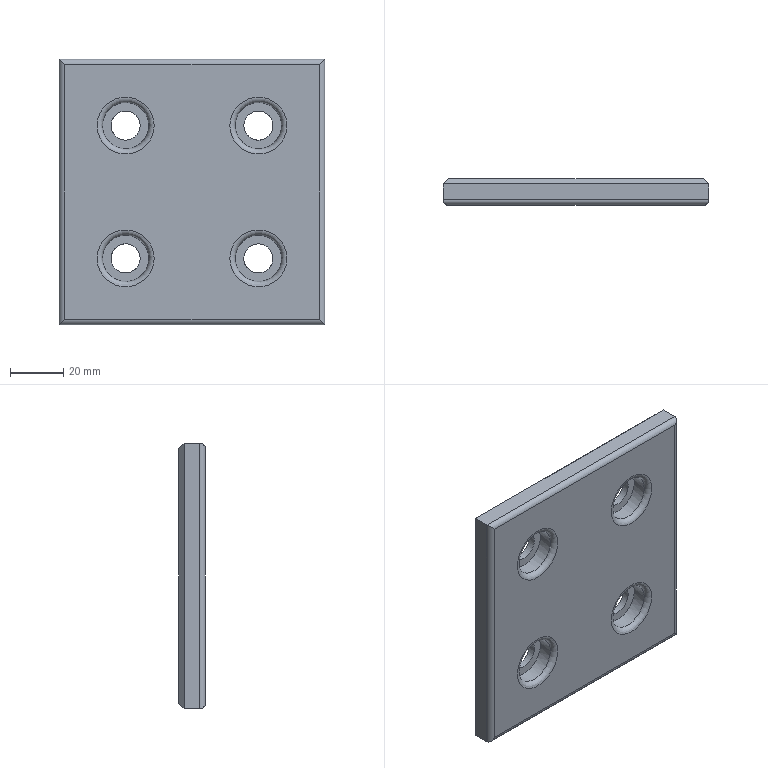Part | NX | features MAIN_BODY 2 | 1 solid | 30 faces | box 100 x 10 x 100 mm | volume 90622 mm3 | plane 14 | cylinder 12 | torus 4 | commonest cylinder face diameters 4 x4 11 x4 17.5 x4
STEP:
#1=CARTESIAN_POINT('',(-666.,240.,-150.5));
#2=VERTEX_POINT('',#1);
#3=CARTESIAN_POINT('',(-570.,240.,-150.5));
#4=VERTEX_POINT('',#3);
#5=CARTESIAN_POINT('',(-568.,240.,-150.5));
#6=DIRECTION('',(-1.,0.,0.));
#7=VECTOR('',#6,1000.);
#8=LINE('',#5,#7);
#9=EDGE_CURVE('',#2,#4,#8,.F.);
#10=ORIENTED_EDGE('',*,*,#9,.T.);
#11=CARTESIAN_POINT('',(-570.,240.,-54.5));
#12=VERTEX_POINT('',#11);
#13=CARTESIAN_POINT('',(-570.,240.,-152.5));
#14=DIRECTION('',(0.,0.,-1.));
#15=VECTOR('',#14,1000.);
#16=LINE('',#13,#15);
#17=EDGE_CURVE('',#4,#12,#16,.F.);
#18=ORIENTED_EDGE('',*,*,#17,.T.);
#19=CARTESIAN_POINT('',(-666.,240.,-54.5));
#20=VERTEX_POINT('',#19);
#21=CARTESIAN_POINT('',(-568.,240.,-54.5));
#22=DIRECTION('',(1.,0.,0.));
#23=VECTOR('',#22,1000.);
#24=LINE('',#21,#23);
#25=EDGE_CURVE('',#12,#20,#24,.F.);
#26=ORIENTED_EDGE('',*,*,#25,.T.);
#27=CARTESIAN_POINT('',(-666.,240.,-152.5));
#28=DIRECTION('',(0.,0.,1.));
#29=VECTOR('',#28,1000.);
#30=LINE('',#27,#29);
#31=EDGE_CURVE('',#20,#2,#30,.F.);
#32=ORIENTED_EDGE('',*,*,#31,.T.);
#33=EDGE_LOOP('',(#10,#18,#26,#32));
#34=FACE_BOUND('',#33,.T.);
#35=CARTESIAN_POINT('',(-582.25,240.,-127.5));
#36=VERTEX_POINT('',#35);
#37=CARTESIAN_POINT('',(-593.,240.,-127.5));
#38=DIRECTION('',(0.,-1.,0.));
#39=DIRECTION('',(1.,0.,0.));
#40=AXIS2_PLACEMENT_3D('',#37,#38,#39);
#41=CIRCLE('',#40,10.75);
#42=EDGE_CURVE('',#36,#36,#41,.F.);
#43=ORIENTED_EDGE('',*,*,#42,.T.);
#44=EDGE_LOOP('',(#43));
#45=FACE_BOUND('',#44,.T.);
#46=CARTESIAN_POINT('',(-582.25,240.,-77.5));
#47=VERTEX_POINT('',#46);
#48=CARTESIAN_POINT('',(-593.,240.,-77.5));
#49=DIRECTION('',(0.,-1.,0.));
#50=DIRECTION('',(1.,0.,0.));
#51=AXIS2_PLACEMENT_3D('',#48,#49,#50);
#52=CIRCLE('',#51,10.75);
#53=EDGE_CURVE('',#47,#47,#52,.F.);
#54=ORIENTED_EDGE('',*,*,#53,.T.);
#55=EDGE_LOOP('',(#54));
#56=FACE_BOUND('',#55,.T.);
#57=CARTESIAN_POINT('',(-632.25,240.,-77.5));
#58=VERTEX_POINT('',#57);
#59=CARTESIAN_POINT('',(-643.,240.,-77.5));
#60=DIRECTION('',(0.,-1.,0.));
#61=DIRECTION('',(1.,0.,0.));
#62=AXIS2_PLACEMENT_3D('',#59,#60,#61);
#63=CIRCLE('',#62,10.75);
#64=EDGE_CURVE('',#58,#58,#63,.F.);
#65=ORIENTED_EDGE('',*,*,#64,.T.);
#66=EDGE_LOOP('',(#65));
#67=FACE_BOUND('',#66,.T.);
#68=CARTESIAN_POINT('',(-632.25,240.,-127.5));
#69=VERTEX_POINT('',#68);
#70=CARTESIAN_POINT('',(-643.,240.,-127.5));
#71=DIRECTION('',(0.,-1.,0.));
#72=DIRECTION('',(1.,0.,0.));
#73=AXIS2_PLACEMENT_3D('',#70,#71,#72);
#74=CIRCLE('',#73,10.75);
#75=EDGE_CURVE('',#69,#69,#74,.F.);
#76=ORIENTED_EDGE('',*,*,#75,.T.);
#77=EDGE_LOOP('',(#76));
#78=FACE_BOUND('',#77,.T.);
#79=CARTESIAN_POINT('',(-568.,240.,-152.5));
#80=DIRECTION('',(0.,-1.,0.));
#81=DIRECTION('',(1.,0.,0.));
#82=AXIS2_PLACEMENT_3D('',#79,#80,#81);
#83=PLANE('',#82);
#84=ADVANCED_FACE('',(#34,#45,#56,#67,#78),#83,.T.);
#85=CARTESIAN_POINT('',(-643.,250.,-83.));
#86=VERTEX_POINT('',#85);
#87=CARTESIAN_POINT('',(-643.,250.,-77.5));
#88=DIRECTION('',(0.,-1.,0.));
#89=DIRECTION('',(0.,0.,-1.));
#90=AXIS2_PLACEMENT_3D('',#87,#88,#89);
#91=CIRCLE('',#90,5.5);
#92=EDGE_CURVE('',#86,#86,#91,.T.);
#93=ORIENTED_EDGE('',*,*,#92,.F.);
#94=EDGE_LOOP('',(#93));
#95=FACE_BOUND('',#94,.T.);
#96=CARTESIAN_POINT('',(-637.5,247.3,-77.5));
#97=VERTEX_POINT('',#96);
#98=CARTESIAN_POINT('',(-643.,247.3,-77.5));
#99=DIRECTION('',(0.,-1.,0.));
#100=DIRECTION('',(1.,0.,0.));
#101=AXIS2_PLACEMENT_3D('',#98,#99,#100);
#102=CIRCLE('',#101,5.5);
#103=EDGE_CURVE('',#97,#97,#102,.T.);
#104=ORIENTED_EDGE('',*,*,#103,.T.);
#105=EDGE_LOOP('',(#104));
#106=FACE_BOUND('',#105,.T.);
#107=CARTESIAN_POINT('',(-643.,230.,-77.5));
#108=DIRECTION('',(0.,1.,0.));
#109=DIRECTION('',(-1.,0.,0.));
#110=AXIS2_PLACEMENT_3D('',#107,#108,#109);
#111=CYLINDRICAL_SURFACE('',#110,5.5);
#112=ADVANCED_FACE('',(#95,#106),#111,.F.);
#113=CARTESIAN_POINT('',(-593.,250.,-122.));
#114=VERTEX_POINT('',#113);
#115=CARTESIAN_POINT('',(-593.,250.,-127.5));
#116=DIRECTION('',(0.,-1.,0.));
#117=DIRECTION('',(0.,0.,1.));
#118=AXIS2_PLACEMENT_3D('',#115,#116,#117);
#119=CIRCLE('',#118,5.5);
#120=EDGE_CURVE('',#114,#114,#119,.T.);
#121=ORIENTED_EDGE('',*,*,#120,.F.);
#122=EDGE_LOOP('',(#121));
#123=FACE_BOUND('',#122,.T.);
#124=CARTESIAN_POINT('',(-587.5,247.3,-127.5));
#125=VERTEX_POINT('',#124);
#126=CARTESIAN_POINT('',(-593.,247.3,-127.5));
#127=DIRECTION('',(0.,-1.,0.));
#128=DIRECTION('',(1.,0.,0.));
#129=AXIS2_PLACEMENT_3D('',#126,#127,#128);
#130=CIRCLE('',#129,5.5);
#131=EDGE_CURVE('',#125,#125,#130,.T.);
#132=ORIENTED_EDGE('',*,*,#131,.T.);
#133=EDGE_LOOP('',(#132));
#134=FACE_BOUND('',#133,.T.);
#135=CARTESIAN_POINT('',(-593.,230.,-127.5));
#136=DIRECTION('',(0.,1.,0.));
#137=DIRECTION('',(-1.,0.,0.));
#138=AXIS2_PLACEMENT_3D('',#135,#136,#137);
#139=CYLINDRICAL_SURFACE('',#138,5.5);
#140=ADVANCED_FACE('',(#123,#134),#139,.F.);
#141=CARTESIAN_POINT('',(-666.,250.,-54.5));
#142=VERTEX_POINT('',#141);
#143=CARTESIAN_POINT('',(-570.,250.,-54.5));
#144=VERTEX_POINT('',#143);
#145=CARTESIAN_POINT('',(-568.,250.,-54.5));
#146=DIRECTION('',(1.,0.,0.));
#147=VECTOR('',#146,1000.);
#148=LINE('',#145,#147);
#149=EDGE_CURVE('',#142,#144,#148,.T.);
#150=ORIENTED_EDGE('',*,*,#149,.T.);
#151=CARTESIAN_POINT('',(-570.,250.,-150.5));
#152=VERTEX_POINT('',#151);
#153=CARTESIAN_POINT('',(-570.,250.,-152.5));
#154=DIRECTION('',(0.,0.,-1.));
#155=VECTOR('',#154,1000.);
#156=LINE('',#153,#155);
#157=EDGE_CURVE('',#144,#152,#156,.T.);
#158=ORIENTED_EDGE('',*,*,#157,.T.);
#159=CARTESIAN_POINT('',(-666.,250.,-150.5));
#160=VERTEX_POINT('',#159);
#161=CARTESIAN_POINT('',(-668.,250.,-150.5));
#162=DIRECTION('',(-1.,0.,0.));
#163=VECTOR('',#162,1000.);
#164=LINE('',#161,#163);
#165=EDGE_CURVE('',#152,#160,#164,.T.);
#166=ORIENTED_EDGE('',*,*,#165,.T.);
#167=CARTESIAN_POINT('',(-666.,250.,-52.5));
#168=DIRECTION('',(0.,0.,1.));
#169=VECTOR('',#168,1000.);
#170=LINE('',#167,#169);
#171=EDGE_CURVE('',#160,#142,#170,.T.);
#172=ORIENTED_EDGE('',*,*,#171,.T.);
#173=EDGE_LOOP('',(#150,#158,#166,#172));
#174=FACE_BOUND('',#173,.T.);
#175=CARTESIAN_POINT('',(-643.,250.,-122.));
#176=VERTEX_POINT('',#175);
#177=CARTESIAN_POINT('',(-643.,250.,-127.5));
#178=DIRECTION('',(0.,1.,0.));
#179=DIRECTION('',(0.,0.,1.));
#180=AXIS2_PLACEMENT_3D('',#177,#178,#179);
#181=CIRCLE('',#180,5.5);
#182=EDGE_CURVE('',#176,#176,#181,.T.);
#183=ORIENTED_EDGE('',*,*,#182,.F.);
#184=EDGE_LOOP('',(#183));
#185=FACE_BOUND('',#184,.T.);
#186=ORIENTED_EDGE('',*,*,#92,.T.);
#187=EDGE_LOOP('',(#186));
#188=FACE_BOUND('',#187,.T.);
#189=CARTESIAN_POINT('',(-593.,250.,-83.));
#190=VERTEX_POINT('',#189);
#191=CARTESIAN_POINT('',(-593.,250.,-77.5));
#192=DIRECTION('',(0.,1.,0.));
#193=DIRECTION('',(0.,0.,-1.));
#194=AXIS2_PLACEMENT_3D('',#191,#192,#193);
#195=CIRCLE('',#194,5.5);
#196=EDGE_CURVE('',#190,#190,#195,.T.);
#197=ORIENTED_EDGE('',*,*,#196,.F.);
#198=EDGE_LOOP('',(#197));
#199=FACE_BOUND('',#198,.T.);
#200=ORIENTED_EDGE('',*,*,#120,.T.);
#201=EDGE_LOOP('',(#200));
#202=FACE_BOUND('',#201,.T.);
#203=CARTESIAN_POINT('',(-568.,250.,-152.5));
#204=DIRECTION('',(0.,-1.,0.));
#205=DIRECTION('',(1.,0.,0.));
#206=AXIS2_PLACEMENT_3D('',#203,#204,#205);
#207=PLANE('',#206);
#208=ADVANCED_FACE('',(#174,#185,#188,#199,#202),#207,.F.);
#209=CARTESIAN_POINT('',(-668.,242.,-152.5));
#210=VERTEX_POINT('',#209);
#211=CARTESIAN_POINT('',(-668.,248.,-152.5));
#212=VERTEX_POINT('',#211);
#213=CARTESIAN_POINT('',(-668.,240.,-152.5));
#214=DIRECTION('',(0.,1.,0.));
#215=VECTOR('',#214,1000.);
#216=LINE('',#213,#215);
#217=EDGE_CURVE('',#210,#212,#216,.T.);
#218=ORIENTED_EDGE('',*,*,#217,.T.);
#219=CARTESIAN_POINT('',(-568.,248.,-152.5));
#220=VERTEX_POINT('',#219);
#221=CARTESIAN_POINT('',(-568.,248.,-152.5));
#222=DIRECTION('',(1.,0.,0.));
#223=VECTOR('',#222,1000.);
#224=LINE('',#221,#223);
#225=EDGE_CURVE('',#212,#220,#224,.T.);
#226=ORIENTED_EDGE('',*,*,#225,.T.);
#227=CARTESIAN_POINT('',(-568.,242.,-152.5));
#228=VERTEX_POINT('',#227);
#229=CARTESIAN_POINT('',(-568.,240.,-152.5));
#230=DIRECTION('',(0.,1.,0.));
#231=VECTOR('',#230,1000.);
#232=LINE('',#229,#231);
#233=EDGE_CURVE('',#228,#220,#232,.T.);
#234=ORIENTED_EDGE('',*,*,#233,.F.);
#235=CARTESIAN_POINT('',(-568.,242.,-152.5));
#236=DIRECTION('',(-1.,0.,0.));
#237=VECTOR('',#236,1000.);
#238=LINE('',#235,#237);
#239=EDGE_CURVE('',#228,#210,#238,.T.);
#240=ORIENTED_EDGE('',*,*,#239,.T.);
#241=EDGE_LOOP('',(#218,#226,#234,#240));
#242=FACE_BOUND('',#241,.T.);
#243=CARTESIAN_POINT('',(-568.,240.,-152.5));
#244=DIRECTION('',(0.,0.,-1.));
#245=DIRECTION('',(1.,0.,0.));
#246=AXIS2_PLACEMENT_3D('',#243,#244,#245);
#247=PLANE('',#246);
#248=ADVANCED_FACE('',(#242),#247,.T.);
#249=CARTESIAN_POINT('',(-668.,242.,-52.5));
#250=VERTEX_POINT('',#249);
#251=CARTESIAN_POINT('',(-668.,248.,-52.5));
#252=VERTEX_POINT('',#251);
#253=CARTESIAN_POINT('',(-668.,240.,-52.5));
#254=DIRECTION('',(0.,1.,0.));
#255=VECTOR('',#254,1000.);
#256=LINE('',#253,#255);
#257=EDGE_CURVE('',#250,#252,#256,.T.);
#258=ORIENTED_EDGE('',*,*,#257,.T.);
#259=CARTESIAN_POINT('',(-668.,248.,-152.5));
#260=DIRECTION('',(0.,0.,-1.));
#261=VECTOR('',#260,1000.);
#262=LINE('',#259,#261);
#263=EDGE_CURVE('',#252,#212,#262,.T.);
#264=ORIENTED_EDGE('',*,*,#263,.T.);
#265=ORIENTED_EDGE('',*,*,#217,.F.);
#266=CARTESIAN_POINT('',(-668.,242.,-152.5));
#267=DIRECTION('',(0.,0.,1.));
#268=VECTOR('',#267,1000.);
#269=LINE('',#266,#268);
#270=EDGE_CURVE('',#210,#250,#269,.T.);
#271=ORIENTED_EDGE('',*,*,#270,.T.);
#272=EDGE_LOOP('',(#258,#264,#265,#271));
#273=FACE_BOUND('',#272,.T.);
#274=CARTESIAN_POINT('',(-668.,240.,-152.5));
#275=DIRECTION('',(-1.,0.,0.));
#276=DIRECTION('',(0.,0.,-1.));
#277=AXIS2_PLACEMENT_3D('',#274,#275,#276);
#278=PLANE('',#277);
#279=ADVANCED_FACE('',(#273),#278,.T.);
#280=CARTESIAN_POINT('',(-568.,242.,-52.5));
#281=VERTEX_POINT('',#280);
#282=CARTESIAN_POINT('',(-568.,248.,-52.5));
#283=VERTEX_POINT('',#282);
#284=CARTESIAN_POINT('',(-568.,240.,-52.5));
#285=DIRECTION('',(0.,1.,0.));
#286=VECTOR('',#285,1000.);
#287=LINE('',#284,#286);
#288=EDGE_CURVE('',#281,#283,#287,.T.);
#289=ORIENTED_EDGE('',*,*,#288,.T.);
#290=CARTESIAN_POINT('',(-668.,248.,-52.5));
#291=DIRECTION('',(-1.,0.,0.));
#292=VECTOR('',#291,1000.);
#293=LINE('',#290,#292);
#294=EDGE_CURVE('',#283,#252,#293,.T.);
#295=ORIENTED_EDGE('',*,*,#294,.T.);
#296=ORIENTED_EDGE('',*,*,#257,.F.);
#297=CARTESIAN_POINT('',(-668.,242.,-52.5));
#298=DIRECTION('',(1.,0.,0.));
#299=VECTOR('',#298,1000.);
#300=LINE('',#297,#299);
#301=EDGE_CURVE('',#250,#281,#300,.T.);
#302=ORIENTED_EDGE('',*,*,#301,.T.);
#303=EDGE_LOOP('',(#289,#295,#296,#302));
#304=FACE_BOUND('',#303,.T.);
#305=CARTESIAN_POINT('',(-668.,240.,-52.5));
#306=DIRECTION('',(0.,0.,1.));
#307=DIRECTION('',(-1.,0.,0.));
#308=AXIS2_PLACEMENT_3D('',#305,#306,#307);
#309=PLANE('',#308);
#310=ADVANCED_FACE('',(#304),#309,.T.);
#311=ORIENTED_EDGE('',*,*,#233,.T.);
#312=CARTESIAN_POINT('',(-568.,248.,-52.5));
#313=DIRECTION('',(0.,0.,1.));
#314=VECTOR('',#313,1000.);
#315=LINE('',#312,#314);
#316=EDGE_CURVE('',#220,#283,#315,.T.);
#317=ORIENTED_EDGE('',*,*,#316,.T.);
#318=ORIENTED_EDGE('',*,*,#288,.F.);
#319=CARTESIAN_POINT('',(-568.,242.,-52.5));
#320=DIRECTION('',(0.,0.,-1.));
#321=VECTOR('',#320,1000.);
#322=LINE('',#319,#321);
#323=EDGE_CURVE('',#281,#228,#322,.T.);
#324=ORIENTED_EDGE('',*,*,#323,.T.);
#325=EDGE_LOOP('',(#311,#317,#318,#324));
#326=FACE_BOUND('',#325,.T.);
#327=CARTESIAN_POINT('',(-568.,240.,-52.5));
#328=DIRECTION('',(1.,0.,0.));
#329=DIRECTION('',(0.,0.,1.));
#330=AXIS2_PLACEMENT_3D('',#327,#328,#329);
#331=PLANE('',#330);
#332=ADVANCED_FACE('',(#326),#331,.T.);
#333=CARTESIAN_POINT('',(-598.5,247.3,-77.5));
#334=VERTEX_POINT('',#333);
#335=CARTESIAN_POINT('',(-593.,247.3,-77.5));
#336=DIRECTION('',(0.,1.,0.));
#337=DIRECTION('',(-1.,0.,0.));
#338=AXIS2_PLACEMENT_3D('',#335,#336,#337);
#339=CIRCLE('',#338,5.5);
#340=EDGE_CURVE('',#334,#334,#339,.F.);
#341=ORIENTED_EDGE('',*,*,#340,.T.);
#342=EDGE_LOOP('',(#341));
#343=FACE_BOUND('',#342,.T.);
#344=ORIENTED_EDGE('',*,*,#196,.T.);
#345=EDGE_LOOP('',(#344));
#346=FACE_BOUND('',#345,.T.);
#347=CARTESIAN_POINT('',(-593.,230.,-77.5));
#348=DIRECTION('',(0.,1.,0.));
#349=DIRECTION('',(-1.,0.,0.));
#350=AXIS2_PLACEMENT_3D('',#347,#348,#349);
#351=CYLINDRICAL_SURFACE('',#350,5.5);
#352=ADVANCED_FACE('',(#343,#346),#351,.F.);
#353=CARTESIAN_POINT('',(-648.5,247.3,-127.5));
#354=VERTEX_POINT('',#353);
#355=CARTESIAN_POINT('',(-643.,247.3,-127.5));
#356=DIRECTION('',(0.,1.,0.));
#357=DIRECTION('',(-1.,0.,0.));
#358=AXIS2_PLACEMENT_3D('',#355,#356,#357);
#359=CIRCLE('',#358,5.5);
#360=EDGE_CURVE('',#354,#354,#359,.F.);
#361=ORIENTED_EDGE('',*,*,#360,.T.);
#362=EDGE_LOOP('',(#361));
#363=FACE_BOUND('',#362,.T.);
#364=ORIENTED_EDGE('',*,*,#182,.T.);
#365=EDGE_LOOP('',(#364));
#366=FACE_BOUND('',#365,.T.);
#367=CARTESIAN_POINT('',(-643.,230.,-127.5));
#368=DIRECTION('',(0.,1.,0.));
#369=DIRECTION('',(-1.,0.,0.));
#370=AXIS2_PLACEMENT_3D('',#367,#368,#369);
#371=CYLINDRICAL_SURFACE('',#370,5.5);
#372=ADVANCED_FACE('',(#363,#366),#371,.F.);
#373=CARTESIAN_POINT('',(-584.25,242.,-127.5));
#374=VERTEX_POINT('',#373);
#375=CARTESIAN_POINT('',(-593.,242.,-127.5));
#376=DIRECTION('',(0.,-1.,0.));
#377=DIRECTION('',(1.,0.,0.));
#378=AXIS2_PLACEMENT_3D('',#375,#376,#377);
#379=CIRCLE('',#378,8.75);
#380=EDGE_CURVE('',#374,#374,#379,.T.);
#381=ORIENTED_EDGE('',*,*,#380,.T.);
#382=EDGE_LOOP('',(#381));
#383=FACE_BOUND('',#382,.T.);
#384=CARTESIAN_POINT('',(-593.,247.3,-118.75));
#385=VERTEX_POINT('',#384);
#386=CARTESIAN_POINT('',(-593.,247.3,-127.5));
#387=DIRECTION('',(0.,-1.,0.));
#388=DIRECTION('',(0.,0.,1.));
#389=AXIS2_PLACEMENT_3D('',#386,#387,#388);
#390=CIRCLE('',#389,8.75);
#391=EDGE_CURVE('',#385,#385,#390,.T.);
#392=ORIENTED_EDGE('',*,*,#391,.F.);
#393=EDGE_LOOP('',(#392));
#394=FACE_BOUND('',#393,.T.);
#395=CARTESIAN_POINT('',(-593.,220.,-127.5));
#396=DIRECTION('',(0.,1.,0.));
#397=DIRECTION('',(-1.,0.,0.));
#398=AXIS2_PLACEMENT_3D('',#395,#396,#397);
#399=CYLINDRICAL_SURFACE('',#398,8.75);
#400=ADVANCED_FACE('',(#383,#394),#399,.F.);
#401=ORIENTED_EDGE('',*,*,#131,.F.);
#402=EDGE_LOOP('',(#401));
#403=FACE_BOUND('',#402,.T.);
#404=ORIENTED_EDGE('',*,*,#391,.T.);
#405=EDGE_LOOP('',(#404));
#406=FACE_BOUND('',#405,.T.);
#407=CARTESIAN_POINT('',(-593.,247.3,-127.5));
#408=DIRECTION('',(0.,-1.,0.));
#409=DIRECTION('',(1.,0.,0.));
#410=AXIS2_PLACEMENT_3D('',#407,#408,#409);
#411=PLANE('',#410);
#412=ADVANCED_FACE('',(#403,#406),#411,.T.);
#413=CARTESIAN_POINT('',(-643.,247.3,-118.75));
#414=VERTEX_POINT('',#413);
#415=CARTESIAN_POINT('',(-643.,247.3,-127.5));
#416=DIRECTION('',(0.,1.,0.));
#417=DIRECTION('',(0.,0.,1.));
#418=AXIS2_PLACEMENT_3D('',#415,#416,#417);
#419=CIRCLE('',#418,8.75);
#420=EDGE_CURVE('',#414,#414,#419,.T.);
#421=ORIENTED_EDGE('',*,*,#420,.F.);
#422=EDGE_LOOP('',(#421));
#423=FACE_BOUND('',#422,.T.);
#424=ORIENTED_EDGE('',*,*,#360,.F.);
#425=EDGE_LOOP('',(#424));
#426=FACE_BOUND('',#425,.T.);
#427=CARTESIAN_POINT('',(-643.,247.3,-127.5));
#428=DIRECTION('',(0.,1.,0.));
#429=DIRECTION('',(-1.,0.,0.));
#430=AXIS2_PLACEMENT_3D('',#427,#428,#429);
#431=PLANE('',#430);
#432=ADVANCED_FACE('',(#423,#426),#431,.F.);
#433=CARTESIAN_POINT('',(-634.25,242.,-127.5));
#434=VERTEX_POINT('',#433);
#435=CARTESIAN_POINT('',(-643.,242.,-127.5));
#436=DIRECTION('',(0.,-1.,0.));
#437=DIRECTION('',(1.,0.,0.));
#438=AXIS2_PLACEMENT_3D('',#435,#436,#437);
#439=CIRCLE('',#438,8.75);
#440=EDGE_CURVE('',#434,#434,#439,.T.);
#441=ORIENTED_EDGE('',*,*,#440,.T.);
#442=EDGE_LOOP('',(#441));
#443=FACE_BOUND('',#442,.T.);
#444=ORIENTED_EDGE('',*,*,#420,.T.);
#445=EDGE_LOOP('',(#444));
#446=FACE_BOUND('',#445,.T.);
#447=CARTESIAN_POINT('',(-643.,220.,-127.5));
#448=DIRECTION('',(0.,1.,0.));
#449=DIRECTION('',(-1.,0.,0.));
#450=AXIS2_PLACEMENT_3D('',#447,#448,#449);
#451=CYLINDRICAL_SURFACE('',#450,8.75);
#452=ADVANCED_FACE('',(#443,#446),#451,.F.);
#453=CARTESIAN_POINT('',(-593.,247.3,-86.25));
#454=VERTEX_POINT('',#453);
#455=CARTESIAN_POINT('',(-593.,247.3,-77.5));
#456=DIRECTION('',(0.,1.,0.));
#457=DIRECTION('',(0.,0.,-1.));
#458=AXIS2_PLACEMENT_3D('',#455,#456,#457);
#459=CIRCLE('',#458,8.75);
#460=EDGE_CURVE('',#454,#454,#459,.T.);
#461=ORIENTED_EDGE('',*,*,#460,.F.);
#462=EDGE_LOOP('',(#461));
#463=FACE_BOUND('',#462,.T.);
#464=ORIENTED_EDGE('',*,*,#340,.F.);
#465=EDGE_LOOP('',(#464));
#466=FACE_BOUND('',#465,.T.);
#467=CARTESIAN_POINT('',(-593.,247.3,-77.5));
#468=DIRECTION('',(0.,1.,0.));
#469=DIRECTION('',(-1.,0.,0.));
#470=AXIS2_PLACEMENT_3D('',#467,#468,#469);
#471=PLANE('',#470);
#472=ADVANCED_FACE('',(#463,#466),#471,.F.);
#473=CARTESIAN_POINT('',(-584.25,242.,-77.5));
#474=VERTEX_POINT('',#473);
#475=CARTESIAN_POINT('',(-593.,242.,-77.5));
#476=DIRECTION('',(0.,-1.,0.));
#477=DIRECTION('',(1.,0.,0.));
#478=AXIS2_PLACEMENT_3D('',#475,#476,#477);
#479=CIRCLE('',#478,8.75);
#480=EDGE_CURVE('',#474,#474,#479,.T.);
#481=ORIENTED_EDGE('',*,*,#480,.T.);
#482=EDGE_LOOP('',(#481));
#483=FACE_BOUND('',#482,.T.);
#484=ORIENTED_EDGE('',*,*,#460,.T.);
#485=EDGE_LOOP('',(#484));
#486=FACE_BOUND('',#485,.T.);
#487=CARTESIAN_POINT('',(-593.,220.,-77.5));
#488=DIRECTION('',(0.,1.,0.));
#489=DIRECTION('',(-1.,0.,0.));
#490=AXIS2_PLACEMENT_3D('',#487,#488,#489);
#491=CYLINDRICAL_SURFACE('',#490,8.75);
#492=ADVANCED_FACE('',(#483,#486),#491,.F.);
#493=CARTESIAN_POINT('',(-634.25,242.,-77.5));
#494=VERTEX_POINT('',#493);
#495=CARTESIAN_POINT('',(-643.,242.,-77.5));
#496=DIRECTION('',(0.,-1.,0.));
#497=DIRECTION('',(1.,0.,0.));
#498=AXIS2_PLACEMENT_3D('',#495,#496,#497);
#499=CIRCLE('',#498,8.75);
#500=EDGE_CURVE('',#494,#494,#499,.T.);
#501=ORIENTED_EDGE('',*,*,#500,.T.);
#502=EDGE_LOOP('',(#501));
#503=FACE_BOUND('',#502,.T.);
#504=CARTESIAN_POINT('',(-643.,247.3,-86.25));
#505=VERTEX_POINT('',#504);
#506=CARTESIAN_POINT('',(-643.,247.3,-77.5));
#507=DIRECTION('',(0.,-1.,0.));
#508=DIRECTION('',(0.,0.,-1.));
#509=AXIS2_PLACEMENT_3D('',#506,#507,#508);
#510=CIRCLE('',#509,8.75);
#511=EDGE_CURVE('',#505,#505,#510,.T.);
#512=ORIENTED_EDGE('',*,*,#511,.F.);
#513=EDGE_LOOP('',(#512));
#514=FACE_BOUND('',#513,.T.);
#515=CARTESIAN_POINT('',(-643.,220.,-77.5));
#516=DIRECTION('',(0.,1.,0.));
#517=DIRECTION('',(-1.,0.,0.));
#518=AXIS2_PLACEMENT_3D('',#515,#516,#517);
#519=CYLINDRICAL_SURFACE('',#518,8.75);
#520=ADVANCED_FACE('',(#503,#514),#519,.F.);
#521=ORIENTED_EDGE('',*,*,#103,.F.);
#522=EDGE_LOOP('',(#521));
#523=FACE_BOUND('',#522,.T.);
#524=ORIENTED_EDGE('',*,*,#511,.T.);
#525=EDGE_LOOP('',(#524));
#526=FACE_BOUND('',#525,.T.);
#527=CARTESIAN_POINT('',(-643.,247.3,-77.5));
#528=DIRECTION('',(0.,-1.,0.));
#529=DIRECTION('',(1.,0.,0.));
#530=AXIS2_PLACEMENT_3D('',#527,#528,#529);
#531=PLANE('',#530);
#532=ADVANCED_FACE('',(#523,#526),#531,.T.);
#533=CARTESIAN_POINT('',(-666.,242.,-150.5));
#534=DIRECTION('',(-0.7071,0.,0.7071));
#535=DIRECTION('',(0.7071,0.,0.7071));
#536=AXIS2_PLACEMENT_3D('',#533,#534,#535);
#537=ELLIPSE('',#536,2.828,2.);
#538=EDGE_CURVE('',#2,#210,#537,.F.);
#539=ORIENTED_EDGE('',*,*,#538,.F.);
#540=ORIENTED_EDGE('',*,*,#31,.F.);
#541=CARTESIAN_POINT('',(-666.,242.,-54.5));
#542=DIRECTION('',(0.7071,0.,0.7071));
#543=DIRECTION('',(-0.7071,0.,0.7071));
#544=AXIS2_PLACEMENT_3D('',#541,#542,#543);
#545=ELLIPSE('',#544,2.828,2.);
#546=EDGE_CURVE('',#250,#20,#545,.T.);
#547=ORIENTED_EDGE('',*,*,#546,.F.);
#548=ORIENTED_EDGE('',*,*,#270,.F.);
#549=EDGE_LOOP('',(#539,#540,#547,#548));
#550=FACE_BOUND('',#549,.T.);
#551=CARTESIAN_POINT('',(-666.,242.,-152.5));
#552=DIRECTION('',(0.,0.,1.));
#553=DIRECTION('',(-1.,0.,0.));
#554=AXIS2_PLACEMENT_3D('',#551,#552,#553);
#555=CYLINDRICAL_SURFACE('',#554,2.);
#556=ADVANCED_FACE('',(#550),#555,.T.);
#557=ORIENTED_EDGE('',*,*,#546,.T.);
#558=ORIENTED_EDGE('',*,*,#25,.F.);
#559=CARTESIAN_POINT('',(-570.,242.,-54.5));
#560=DIRECTION('',(0.7071,0.,-0.7071));
#561=DIRECTION('',(0.7071,0.,0.7071));
#562=AXIS2_PLACEMENT_3D('',#559,#560,#561);
#563=ELLIPSE('',#562,2.828,2.);
#564=EDGE_CURVE('',#281,#12,#563,.T.);
#565=ORIENTED_EDGE('',*,*,#564,.F.);
#566=ORIENTED_EDGE('',*,*,#301,.F.);
#567=EDGE_LOOP('',(#557,#558,#565,#566));
#568=FACE_BOUND('',#567,.T.);
#569=CARTESIAN_POINT('',(-668.,242.,-54.5));
#570=DIRECTION('',(1.,0.,0.));
#571=DIRECTION('',(0.,0.,1.));
#572=AXIS2_PLACEMENT_3D('',#569,#570,#571);
#573=CYLINDRICAL_SURFACE('',#572,2.);
#574=ADVANCED_FACE('',(#568),#573,.T.);
#575=ORIENTED_EDGE('',*,*,#538,.T.);
#576=ORIENTED_EDGE('',*,*,#239,.F.);
#577=CARTESIAN_POINT('',(-570.,242.,-150.5));
#578=DIRECTION('',(-0.7071,0.,-0.7071));
#579=DIRECTION('',(-0.7071,0.,0.7071));
#580=AXIS2_PLACEMENT_3D('',#577,#578,#579);
#581=ELLIPSE('',#580,2.828,2.);
#582=EDGE_CURVE('',#4,#228,#581,.F.);
#583=ORIENTED_EDGE('',*,*,#582,.F.);
#584=ORIENTED_EDGE('',*,*,#9,.F.);
#585=EDGE_LOOP('',(#575,#576,#583,#584));
#586=FACE_BOUND('',#585,.T.);
#587=CARTESIAN_POINT('',(-568.,242.,-150.5));
#588=DIRECTION('',(-1.,0.,0.));
#589=DIRECTION('',(0.,0.,-1.));
#590=AXIS2_PLACEMENT_3D('',#587,#588,#589);
#591=CYLINDRICAL_SURFACE('',#590,2.);
#592=ADVANCED_FACE('',(#586),#591,.T.);
#593=ORIENTED_EDGE('',*,*,#564,.T.);
#594=ORIENTED_EDGE('',*,*,#17,.F.);
#595=ORIENTED_EDGE('',*,*,#582,.T.);
#596=ORIENTED_EDGE('',*,*,#323,.F.);
#597=EDGE_LOOP('',(#593,#594,#595,#596));
#598=FACE_BOUND('',#597,.T.);
#599=CARTESIAN_POINT('',(-570.,242.,-52.5));
#600=DIRECTION('',(0.,0.,-1.));
#601=DIRECTION('',(1.,0.,0.));
#602=AXIS2_PLACEMENT_3D('',#599,#600,#601);
#603=CYLINDRICAL_SURFACE('',#602,2.);
#604=ADVANCED_FACE('',(#598),#603,.T.);
#605=ORIENTED_EDGE('',*,*,#380,.F.);
#606=EDGE_LOOP('',(#605));
#607=FACE_BOUND('',#606,.T.);
#608=ORIENTED_EDGE('',*,*,#42,.F.);
#609=EDGE_LOOP('',(#608));
#610=FACE_BOUND('',#609,.T.);
#611=CARTESIAN_POINT('',(-593.,242.,-127.5));
#612=DIRECTION('',(0.,-1.,0.));
#613=DIRECTION('',(1.,0.,0.));
#614=AXIS2_PLACEMENT_3D('',#611,#612,#613);
#615=TOROIDAL_SURFACE('',#614,10.75,2.);
#616=ADVANCED_FACE('',(#607,#610),#615,.T.);
#617=ORIENTED_EDGE('',*,*,#53,.F.);
#618=EDGE_LOOP('',(#617));
#619=FACE_BOUND('',#618,.T.);
#620=ORIENTED_EDGE('',*,*,#480,.F.);
#621=EDGE_LOOP('',(#620));
#622=FACE_BOUND('',#621,.T.);
#623=CARTESIAN_POINT('',(-593.,242.,-77.5));
#624=DIRECTION('',(0.,-1.,0.));
#625=DIRECTION('',(1.,0.,0.));
#626=AXIS2_PLACEMENT_3D('',#623,#624,#625);
#627=TOROIDAL_SURFACE('',#626,10.75,2.);
#628=ADVANCED_FACE('',(#619,#622),#627,.T.);
#629=ORIENTED_EDGE('',*,*,#500,.F.);
#630=EDGE_LOOP('',(#629));
#631=FACE_BOUND('',#630,.T.);
#632=ORIENTED_EDGE('',*,*,#64,.F.);
#633=EDGE_LOOP('',(#632));
#634=FACE_BOUND('',#633,.T.);
#635=CARTESIAN_POINT('',(-643.,242.,-77.5));
#636=DIRECTION('',(0.,-1.,0.));
#637=DIRECTION('',(1.,0.,0.));
#638=AXIS2_PLACEMENT_3D('',#635,#636,#637);
#639=TOROIDAL_SURFACE('',#638,10.75,2.);
#640=ADVANCED_FACE('',(#631,#634),#639,.T.);
#641=ORIENTED_EDGE('',*,*,#75,.F.);
#642=EDGE_LOOP('',(#641));
#643=FACE_BOUND('',#642,.T.);
#644=ORIENTED_EDGE('',*,*,#440,.F.);
#645=EDGE_LOOP('',(#644));
#646=FACE_BOUND('',#645,.T.);
#647=CARTESIAN_POINT('',(-643.,242.,-127.5));
#648=DIRECTION('',(0.,-1.,0.));
#649=DIRECTION('',(1.,0.,0.));
#650=AXIS2_PLACEMENT_3D('',#647,#648,#649);
#651=TOROIDAL_SURFACE('',#650,10.75,2.);
#652=ADVANCED_FACE('',(#643,#646),#651,.T.);
#653=CARTESIAN_POINT('',(-666.667,249.333,-151.167));
#654=DIRECTION('',(-0.5774,-0.5774,-0.5774));
#655=VECTOR('',#654,1000.);
#656=LINE('',#653,#655);
#657=EDGE_CURVE('',#212,#160,#656,.F.);
#658=ORIENTED_EDGE('',*,*,#657,.F.);
#659=ORIENTED_EDGE('',*,*,#263,.F.);
#660=CARTESIAN_POINT('',(-633.333,282.667,-87.167));
#661=DIRECTION('',(-0.5774,-0.5774,0.5774));
#662=VECTOR('',#661,1000.);
#663=LINE('',#660,#662);
#664=EDGE_CURVE('',#142,#252,#663,.T.);
#665=ORIENTED_EDGE('',*,*,#664,.F.);
#666=ORIENTED_EDGE('',*,*,#171,.F.);
#667=EDGE_LOOP('',(#658,#659,#665,#666));
#668=FACE_BOUND('',#667,.T.);
#669=CARTESIAN_POINT('',(-666.,250.,-152.5));
#670=DIRECTION('',(-0.7071,0.7071,0.));
#671=DIRECTION('',(-0.7071,-0.7071,0.));
#672=AXIS2_PLACEMENT_3D('',#669,#670,#671);
#673=PLANE('',#672);
#674=ADVANCED_FACE('',(#668),#673,.T.);
#675=ORIENTED_EDGE('',*,*,#664,.T.);
#676=ORIENTED_EDGE('',*,*,#294,.F.);
#677=CARTESIAN_POINT('',(-569.333,249.333,-53.833));
#678=DIRECTION('',(-0.5774,0.5774,-0.5774));
#679=VECTOR('',#678,1000.);
#680=LINE('',#677,#679);
#681=EDGE_CURVE('',#144,#283,#680,.F.);
#682=ORIENTED_EDGE('',*,*,#681,.F.);
#683=ORIENTED_EDGE('',*,*,#149,.F.);
#684=EDGE_LOOP('',(#675,#676,#682,#683));
#685=FACE_BOUND('',#684,.T.);
#686=CARTESIAN_POINT('',(-568.,250.,-54.5));
#687=DIRECTION('',(0.,0.7071,0.7071));
#688=DIRECTION('',(0.,0.7071,-0.7071));
#689=AXIS2_PLACEMENT_3D('',#686,#687,#688);
#690=PLANE('',#689);
#691=ADVANCED_FACE('',(#685),#690,.T.);
#692=ORIENTED_EDGE('',*,*,#657,.T.);
#693=ORIENTED_EDGE('',*,*,#165,.F.);
#694=CARTESIAN_POINT('',(-569.333,249.333,-151.167));
#695=DIRECTION('',(0.5774,-0.5774,-0.5774));
#696=VECTOR('',#695,1000.);
#697=LINE('',#694,#696);
#698=EDGE_CURVE('',#220,#152,#697,.F.);
#699=ORIENTED_EDGE('',*,*,#698,.F.);
#700=ORIENTED_EDGE('',*,*,#225,.F.);
#701=EDGE_LOOP('',(#692,#693,#699,#700));
#702=FACE_BOUND('',#701,.T.);
#703=CARTESIAN_POINT('',(-568.,250.,-150.5));
#704=DIRECTION('',(0.,0.7071,-0.7071));
#705=DIRECTION('',(0.,-0.7071,-0.7071));
#706=AXIS2_PLACEMENT_3D('',#703,#704,#705);
#707=PLANE('',#706);
#708=ADVANCED_FACE('',(#702),#707,.T.);
#709=ORIENTED_EDGE('',*,*,#681,.T.);
#710=ORIENTED_EDGE('',*,*,#316,.F.);
#711=ORIENTED_EDGE('',*,*,#698,.T.);
#712=ORIENTED_EDGE('',*,*,#157,.F.);
#713=EDGE_LOOP('',(#709,#710,#711,#712));
#714=FACE_BOUND('',#713,.T.);
#715=CARTESIAN_POINT('',(-570.,250.,-152.5));
#716=DIRECTION('',(0.7071,0.7071,0.));
#717=DIRECTION('',(-0.7071,0.7071,0.));
#718=AXIS2_PLACEMENT_3D('',#715,#716,#717);
#719=PLANE('',#718);
#720=ADVANCED_FACE('',(#714),#719,.T.);
#721=CLOSED_SHELL('',(#84,#112,#140,#208,#248,#279,#310,#332,#352,#372,#400,#412,#432,#452,#472,#492,#520,#532,#556,#574,#592,#604,#616,#628,#640,#652,#674,#691,#708,#720));
#722=MANIFOLD_SOLID_BREP('',#721);
#723=(LENGTH_UNIT()NAMED_UNIT(*)SI_UNIT(.MILLI.,.METRE.));
#724=UNCERTAINTY_MEASURE_WITH_UNIT(LENGTH_MEASURE(0.00001),#723,'','');
#725=(NAMED_UNIT(*)PLANE_ANGLE_UNIT()SI_UNIT($,.RADIAN.));
#726=(NAMED_UNIT(*)SI_UNIT($,.STERADIAN.)SOLID_ANGLE_UNIT());
#727=(GEOMETRIC_REPRESENTATION_CONTEXT(3)GLOBAL_UNCERTAINTY_ASSIGNED_CONTEXT((#724))GLOBAL_UNIT_ASSIGNED_CONTEXT((#723,#725,#726))REPRESENTATION_CONTEXT('',''));
#728=ADVANCED_BREP_SHAPE_REPRESENTATION('',(#722),#727);